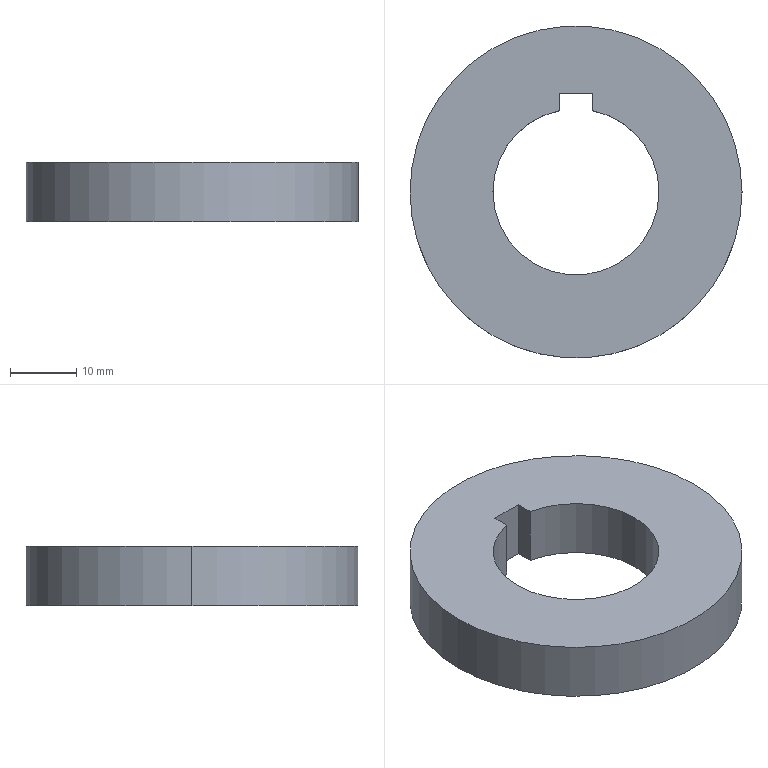Part | SolidWorks | features Extrusion 1, ICE 1, MoveFace 1 | 1 solid | 10 faces | box 50 x 50 x 9.018 mm | volume 13173 mm3 | cylinder 5 | plane 5 | commonest cylinder face diameters 25 x3 50 x2
STEP:
#1=CARTESIAN_POINT('',(-12.5,0.,-17.));
#2=VERTEX_POINT('',#1);
#3=CARTESIAN_POINT('',(12.5,0.,-17.));
#4=VERTEX_POINT('',#3);
#5=CARTESIAN_POINT('',(0.,0.,-17.));
#6=DIRECTION('',(0.,0.,1.));
#7=DIRECTION('',(1.,0.,0.));
#8=AXIS2_PLACEMENT_3D('',#5,#6,#7);
#9=CIRCLE('',#8,12.5);
#10=EDGE_CURVE('',#2,#4,#9,.T.);
#11=ORIENTED_EDGE('',*,*,#10,.F.);
#12=CARTESIAN_POINT('',(-12.5,0.,-7.982));
#13=VERTEX_POINT('',#12);
#14=CARTESIAN_POINT('',(-12.5,0.,-17.));
#15=DIRECTION('',(0.,0.,1.));
#16=VECTOR('',#15,1000.);
#17=LINE('',#14,#16);
#18=EDGE_CURVE('',#2,#13,#17,.T.);
#19=ORIENTED_EDGE('',*,*,#18,.T.);
#20=CARTESIAN_POINT('',(12.5,0.,-7.982));
#21=VERTEX_POINT('',#20);
#22=CARTESIAN_POINT('',(0.,0.,-7.982));
#23=DIRECTION('',(0.,0.,1.));
#24=DIRECTION('',(1.,0.,0.));
#25=AXIS2_PLACEMENT_3D('',#22,#23,#24);
#26=CIRCLE('',#25,12.5);
#27=EDGE_CURVE('',#13,#21,#26,.T.);
#28=ORIENTED_EDGE('',*,*,#27,.T.);
#29=CARTESIAN_POINT('',(12.5,0.,-17.));
#30=DIRECTION('',(0.,0.,1.));
#31=VECTOR('',#30,1000.);
#32=LINE('',#29,#31);
#33=EDGE_CURVE('',#4,#21,#32,.T.);
#34=ORIENTED_EDGE('',*,*,#33,.F.);
#35=EDGE_LOOP('',(#11,#19,#28,#34));
#36=FACE_OUTER_BOUND('',#35,.T.);
#37=CARTESIAN_POINT('',(0.,0.,-17.));
#38=DIRECTION('',(0.,0.,1.));
#39=DIRECTION('',(1.,0.,0.));
#40=AXIS2_PLACEMENT_3D('',#37,#38,#39);
#41=CYLINDRICAL_SURFACE('',#40,12.5);
#42=ADVANCED_FACE('',(#36),#41,.F.);
#43=CARTESIAN_POINT('',(2.5,12.247,-17.));
#44=VERTEX_POINT('',#43);
#45=CARTESIAN_POINT('',(0.,0.,-17.));
#46=DIRECTION('',(0.,0.,1.));
#47=DIRECTION('',(1.,0.,0.));
#48=AXIS2_PLACEMENT_3D('',#45,#46,#47);
#49=CIRCLE('',#48,12.5);
#50=EDGE_CURVE('',#4,#44,#49,.T.);
#51=ORIENTED_EDGE('',*,*,#50,.F.);
#52=ORIENTED_EDGE('',*,*,#33,.T.);
#53=CARTESIAN_POINT('',(2.5,12.247,-7.982));
#54=VERTEX_POINT('',#53);
#55=CARTESIAN_POINT('',(0.,0.,-7.982));
#56=DIRECTION('',(0.,0.,1.));
#57=DIRECTION('',(1.,0.,0.));
#58=AXIS2_PLACEMENT_3D('',#55,#56,#57);
#59=CIRCLE('',#58,12.5);
#60=EDGE_CURVE('',#21,#54,#59,.T.);
#61=ORIENTED_EDGE('',*,*,#60,.T.);
#62=CARTESIAN_POINT('',(2.5,12.247,-17.));
#63=DIRECTION('',(0.,0.,-1.));
#64=VECTOR('',#63,1000.);
#65=LINE('',#62,#64);
#66=EDGE_CURVE('',#54,#44,#65,.T.);
#67=ORIENTED_EDGE('',*,*,#66,.T.);
#68=EDGE_LOOP('',(#51,#52,#61,#67));
#69=FACE_OUTER_BOUND('',#68,.T.);
#70=CARTESIAN_POINT('',(0.,0.,-17.));
#71=DIRECTION('',(0.,0.,1.));
#72=DIRECTION('',(1.,0.,0.));
#73=AXIS2_PLACEMENT_3D('',#70,#71,#72);
#74=CYLINDRICAL_SURFACE('',#73,12.5);
#75=ADVANCED_FACE('',(#69),#74,.F.);
#76=CARTESIAN_POINT('',(25.,0.,-17.));
#77=VERTEX_POINT('',#76);
#78=CARTESIAN_POINT('',(-25.,0.,-17.));
#79=VERTEX_POINT('',#78);
#80=CARTESIAN_POINT('',(0.,0.,-17.));
#81=DIRECTION('',(0.,0.,1.));
#82=DIRECTION('',(1.,0.,0.));
#83=AXIS2_PLACEMENT_3D('',#80,#81,#82);
#84=CIRCLE('',#83,25.);
#85=EDGE_CURVE('',#77,#79,#84,.T.);
#86=ORIENTED_EDGE('',*,*,#85,.T.);
#87=CARTESIAN_POINT('',(-25.,0.,-7.982));
#88=VERTEX_POINT('',#87);
#89=CARTESIAN_POINT('',(-25.,0.,-17.));
#90=DIRECTION('',(0.,0.,1.));
#91=VECTOR('',#90,1000.);
#92=LINE('',#89,#91);
#93=EDGE_CURVE('',#79,#88,#92,.T.);
#94=ORIENTED_EDGE('',*,*,#93,.T.);
#95=CARTESIAN_POINT('',(25.,0.,-7.982));
#96=VERTEX_POINT('',#95);
#97=CARTESIAN_POINT('',(0.,0.,-7.982));
#98=DIRECTION('',(0.,0.,1.));
#99=DIRECTION('',(1.,0.,0.));
#100=AXIS2_PLACEMENT_3D('',#97,#98,#99);
#101=CIRCLE('',#100,25.);
#102=EDGE_CURVE('',#96,#88,#101,.T.);
#103=ORIENTED_EDGE('',*,*,#102,.F.);
#104=CARTESIAN_POINT('',(25.,0.,-17.));
#105=DIRECTION('',(0.,0.,1.));
#106=VECTOR('',#105,1000.);
#107=LINE('',#104,#106);
#108=EDGE_CURVE('',#77,#96,#107,.T.);
#109=ORIENTED_EDGE('',*,*,#108,.F.);
#110=EDGE_LOOP('',(#86,#94,#103,#109));
#111=FACE_OUTER_BOUND('',#110,.T.);
#112=CARTESIAN_POINT('',(0.,0.,-17.));
#113=DIRECTION('',(0.,0.,1.));
#114=DIRECTION('',(1.,0.,0.));
#115=AXIS2_PLACEMENT_3D('',#112,#113,#114);
#116=CYLINDRICAL_SURFACE('',#115,25.);
#117=ADVANCED_FACE('',(#111),#116,.T.);
#118=ORIENTED_EDGE('',*,*,#93,.F.);
#119=CARTESIAN_POINT('',(0.,0.,-17.));
#120=DIRECTION('',(0.,0.,1.));
#121=DIRECTION('',(1.,0.,0.));
#122=AXIS2_PLACEMENT_3D('',#119,#120,#121);
#123=CIRCLE('',#122,25.);
#124=EDGE_CURVE('',#79,#77,#123,.T.);
#125=ORIENTED_EDGE('',*,*,#124,.T.);
#126=ORIENTED_EDGE('',*,*,#108,.T.);
#127=CARTESIAN_POINT('',(0.,0.,-7.982));
#128=DIRECTION('',(0.,0.,1.));
#129=DIRECTION('',(1.,0.,0.));
#130=AXIS2_PLACEMENT_3D('',#127,#128,#129);
#131=CIRCLE('',#130,25.);
#132=EDGE_CURVE('',#88,#96,#131,.T.);
#133=ORIENTED_EDGE('',*,*,#132,.F.);
#134=EDGE_LOOP('',(#118,#125,#126,#133));
#135=FACE_OUTER_BOUND('',#134,.T.);
#136=CARTESIAN_POINT('',(0.,0.,-17.));
#137=DIRECTION('',(0.,0.,1.));
#138=DIRECTION('',(1.,0.,0.));
#139=AXIS2_PLACEMENT_3D('',#136,#137,#138);
#140=CYLINDRICAL_SURFACE('',#139,25.);
#141=ADVANCED_FACE('',(#135),#140,.T.);
#142=CARTESIAN_POINT('',(-2.5,14.8,-17.));
#143=VERTEX_POINT('',#142);
#144=CARTESIAN_POINT('',(2.5,14.8,-17.));
#145=VERTEX_POINT('',#144);
#146=CARTESIAN_POINT('',(2.5,14.8,-17.));
#147=DIRECTION('',(1.,0.,0.));
#148=VECTOR('',#147,1000.);
#149=LINE('',#146,#148);
#150=EDGE_CURVE('',#143,#145,#149,.T.);
#151=ORIENTED_EDGE('',*,*,#150,.F.);
#152=CARTESIAN_POINT('',(-2.5,12.247,-17.));
#153=VERTEX_POINT('',#152);
#154=CARTESIAN_POINT('',(-2.5,10.2,-17.));
#155=DIRECTION('',(0.,1.,0.));
#156=VECTOR('',#155,1000.);
#157=LINE('',#154,#156);
#158=EDGE_CURVE('',#153,#143,#157,.T.);
#159=ORIENTED_EDGE('',*,*,#158,.F.);
#160=CARTESIAN_POINT('',(0.,0.,-17.));
#161=DIRECTION('',(0.,0.,1.));
#162=DIRECTION('',(1.,0.,0.));
#163=AXIS2_PLACEMENT_3D('',#160,#161,#162);
#164=CIRCLE('',#163,12.5);
#165=EDGE_CURVE('',#153,#2,#164,.T.);
#166=ORIENTED_EDGE('',*,*,#165,.T.);
#167=ORIENTED_EDGE('',*,*,#10,.T.);
#168=ORIENTED_EDGE('',*,*,#50,.T.);
#169=CARTESIAN_POINT('',(2.5,10.2,-17.));
#170=DIRECTION('',(0.,-1.,0.));
#171=VECTOR('',#170,1000.);
#172=LINE('',#169,#171);
#173=EDGE_CURVE('',#145,#44,#172,.T.);
#174=ORIENTED_EDGE('',*,*,#173,.F.);
#175=EDGE_LOOP('',(#151,#159,#166,#167,#168,#174));
#176=FACE_BOUND('',#175,.T.);
#177=ORIENTED_EDGE('',*,*,#85,.F.);
#178=ORIENTED_EDGE('',*,*,#124,.F.);
#179=EDGE_LOOP('',(#177,#178));
#180=FACE_OUTER_BOUND('',#179,.T.);
#181=CARTESIAN_POINT('',(0.,0.,-17.));
#182=DIRECTION('',(0.,0.,1.));
#183=DIRECTION('',(1.,0.,0.));
#184=AXIS2_PLACEMENT_3D('',#181,#182,#183);
#185=PLANE('',#184);
#186=ADVANCED_FACE('',(#176,#180),#185,.F.);
#187=CARTESIAN_POINT('',(-2.5,12.247,-7.982));
#188=VERTEX_POINT('',#187);
#189=CARTESIAN_POINT('',(-2.5,14.8,-7.982));
#190=VERTEX_POINT('',#189);
#191=CARTESIAN_POINT('',(-2.5,10.2,-7.982));
#192=DIRECTION('',(0.,1.,0.));
#193=VECTOR('',#192,1000.);
#194=LINE('',#191,#193);
#195=EDGE_CURVE('',#188,#190,#194,.T.);
#196=ORIENTED_EDGE('',*,*,#195,.T.);
#197=CARTESIAN_POINT('',(2.5,14.8,-7.982));
#198=VERTEX_POINT('',#197);
#199=CARTESIAN_POINT('',(2.5,14.8,-7.982));
#200=DIRECTION('',(1.,0.,0.));
#201=VECTOR('',#200,1000.);
#202=LINE('',#199,#201);
#203=EDGE_CURVE('',#190,#198,#202,.T.);
#204=ORIENTED_EDGE('',*,*,#203,.T.);
#205=CARTESIAN_POINT('',(2.5,10.2,-7.982));
#206=DIRECTION('',(0.,-1.,0.));
#207=VECTOR('',#206,1000.);
#208=LINE('',#205,#207);
#209=EDGE_CURVE('',#198,#54,#208,.T.);
#210=ORIENTED_EDGE('',*,*,#209,.T.);
#211=ORIENTED_EDGE('',*,*,#60,.F.);
#212=ORIENTED_EDGE('',*,*,#27,.F.);
#213=CARTESIAN_POINT('',(0.,0.,-7.982));
#214=DIRECTION('',(0.,0.,1.));
#215=DIRECTION('',(1.,0.,0.));
#216=AXIS2_PLACEMENT_3D('',#213,#214,#215);
#217=CIRCLE('',#216,12.5);
#218=EDGE_CURVE('',#188,#13,#217,.T.);
#219=ORIENTED_EDGE('',*,*,#218,.F.);
#220=EDGE_LOOP('',(#196,#204,#210,#211,#212,#219));
#221=FACE_BOUND('',#220,.T.);
#222=ORIENTED_EDGE('',*,*,#102,.T.);
#223=ORIENTED_EDGE('',*,*,#132,.T.);
#224=EDGE_LOOP('',(#222,#223));
#225=FACE_OUTER_BOUND('',#224,.T.);
#226=CARTESIAN_POINT('',(0.,0.,-7.982));
#227=DIRECTION('',(0.,0.,1.));
#228=DIRECTION('',(1.,0.,0.));
#229=AXIS2_PLACEMENT_3D('',#226,#227,#228);
#230=PLANE('',#229);
#231=ADVANCED_FACE('',(#221,#225),#230,.T.);
#232=ORIENTED_EDGE('',*,*,#18,.F.);
#233=ORIENTED_EDGE('',*,*,#165,.F.);
#234=CARTESIAN_POINT('',(-2.5,12.247,-17.));
#235=DIRECTION('',(0.,0.,1.));
#236=VECTOR('',#235,1000.);
#237=LINE('',#234,#236);
#238=EDGE_CURVE('',#153,#188,#237,.T.);
#239=ORIENTED_EDGE('',*,*,#238,.T.);
#240=ORIENTED_EDGE('',*,*,#218,.T.);
#241=EDGE_LOOP('',(#232,#233,#239,#240));
#242=FACE_OUTER_BOUND('',#241,.T.);
#243=CARTESIAN_POINT('',(0.,0.,-17.));
#244=DIRECTION('',(0.,0.,1.));
#245=DIRECTION('',(1.,0.,0.));
#246=AXIS2_PLACEMENT_3D('',#243,#244,#245);
#247=CYLINDRICAL_SURFACE('',#246,12.5);
#248=ADVANCED_FACE('',(#242),#247,.F.);
#249=ORIENTED_EDGE('',*,*,#158,.T.);
#250=CARTESIAN_POINT('',(-2.5,14.8,-7.982));
#251=DIRECTION('',(0.,0.,-1.));
#252=VECTOR('',#251,1000.);
#253=LINE('',#250,#252);
#254=EDGE_CURVE('',#190,#143,#253,.T.);
#255=ORIENTED_EDGE('',*,*,#254,.F.);
#256=ORIENTED_EDGE('',*,*,#195,.F.);
#257=ORIENTED_EDGE('',*,*,#238,.F.);
#258=EDGE_LOOP('',(#249,#255,#256,#257));
#259=FACE_OUTER_BOUND('',#258,.T.);
#260=CARTESIAN_POINT('',(-2.5,10.2,-7.982));
#261=DIRECTION('',(-1.,0.,0.));
#262=DIRECTION('',(0.,0.,1.));
#263=AXIS2_PLACEMENT_3D('',#260,#261,#262);
#264=PLANE('',#263);
#265=ADVANCED_FACE('',(#259),#264,.F.);
#266=ORIENTED_EDGE('',*,*,#209,.F.);
#267=CARTESIAN_POINT('',(2.5,14.8,-7.982));
#268=DIRECTION('',(0.,0.,-1.));
#269=VECTOR('',#268,1000.);
#270=LINE('',#267,#269);
#271=EDGE_CURVE('',#198,#145,#270,.T.);
#272=ORIENTED_EDGE('',*,*,#271,.T.);
#273=ORIENTED_EDGE('',*,*,#173,.T.);
#274=ORIENTED_EDGE('',*,*,#66,.F.);
#275=EDGE_LOOP('',(#266,#272,#273,#274));
#276=FACE_OUTER_BOUND('',#275,.T.);
#277=CARTESIAN_POINT('',(2.5,10.2,-7.982));
#278=DIRECTION('',(1.,0.,0.));
#279=DIRECTION('',(0.,0.,-1.));
#280=AXIS2_PLACEMENT_3D('',#277,#278,#279);
#281=PLANE('',#280);
#282=ADVANCED_FACE('',(#276),#281,.F.);
#283=ORIENTED_EDGE('',*,*,#150,.T.);
#284=ORIENTED_EDGE('',*,*,#271,.F.);
#285=ORIENTED_EDGE('',*,*,#203,.F.);
#286=ORIENTED_EDGE('',*,*,#254,.T.);
#287=EDGE_LOOP('',(#283,#284,#285,#286));
#288=FACE_OUTER_BOUND('',#287,.T.);
#289=CARTESIAN_POINT('',(2.5,14.8,-7.982));
#290=DIRECTION('',(0.,1.,0.));
#291=DIRECTION('',(0.,0.,1.));
#292=AXIS2_PLACEMENT_3D('',#289,#290,#291);
#293=PLANE('',#292);
#294=ADVANCED_FACE('',(#288),#293,.F.);
#295=CLOSED_SHELL('',(#42,#75,#117,#141,#186,#231,#248,#265,#282,#294));
#296=MANIFOLD_SOLID_BREP('',#295);
#297=CARTESIAN_POINT('',(0.,0.,0.));
#298=DIRECTION('',(0.,0.,1.));
#299=DIRECTION('',(1.,0.,0.));
#300=AXIS2_PLACEMENT_3D('',#297,#298,#299);
#301=(LENGTH_UNIT()NAMED_UNIT(*)SI_UNIT(.MILLI.,.METRE.));
#302=UNCERTAINTY_MEASURE_WITH_UNIT(LENGTH_MEASURE(0.00001),#301,'','');
#303=(NAMED_UNIT(*)PLANE_ANGLE_UNIT()SI_UNIT($,.RADIAN.));
#304=(NAMED_UNIT(*)SI_UNIT($,.STERADIAN.)SOLID_ANGLE_UNIT());
#305=(GEOMETRIC_REPRESENTATION_CONTEXT(3)GLOBAL_UNCERTAINTY_ASSIGNED_CONTEXT((#302))GLOBAL_UNIT_ASSIGNED_CONTEXT((#301,#303,#304))REPRESENTATION_CONTEXT('',''));
#306=ADVANCED_BREP_SHAPE_REPRESENTATION('',(#296,#300),#305);